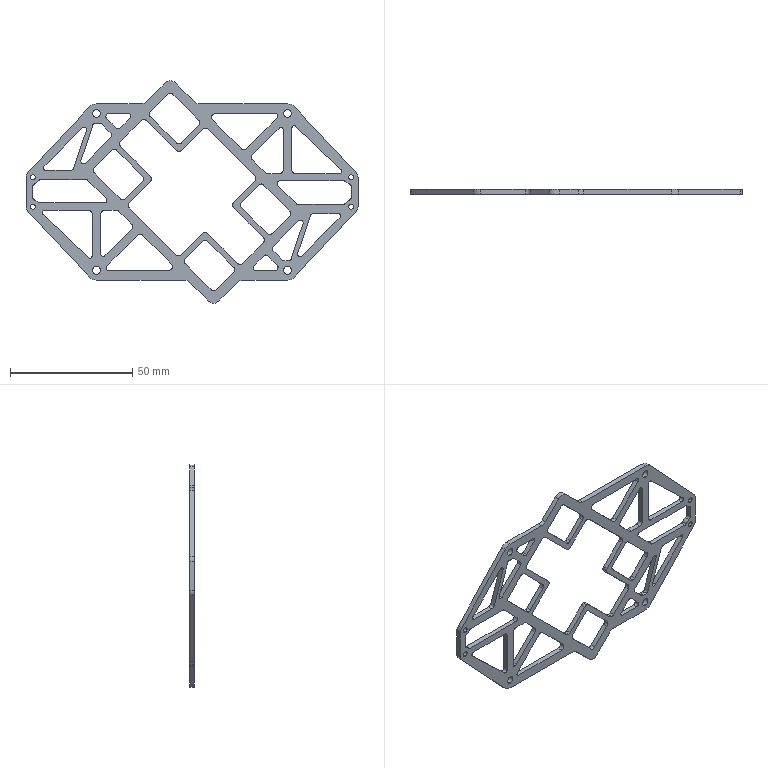Part | SolidWorks | features Fillet 3, Extrusion 1, ICE 1 | 1 solid | 235 faces | box 135.6 x 2 x 90.853 mm | volume 6413 mm3 | cylinder 145 | plane 90 | commonest cylinder face diameters 3 x53 2 x50 8 x11 2.1 x8 3.1 x8 5.6 x8